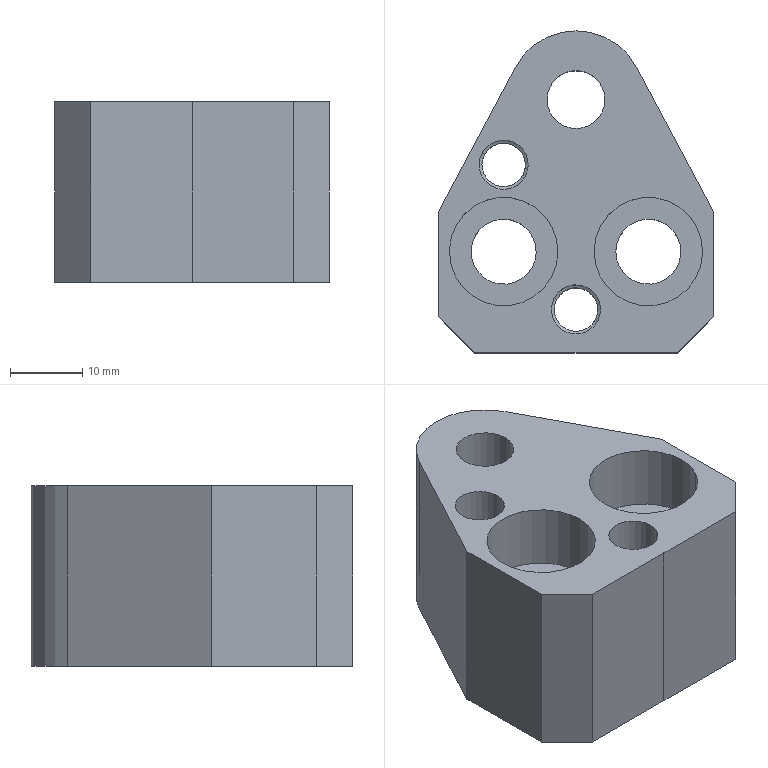Part | CATIA | 1 solid | 39 faces | box 38 x 44.5 x 25 mm | volume 24726 mm3 | cylinder 22 | plane 13 | cone 4 | commonest cylinder face diameters 6 x4 6.8 x4 9 x4 15 x4 8 x2 12 x2
STEP:
#1=CARTESIAN_POINT('',(2.984,-30.63,25.));
#2=VERTEX_POINT('',#1);
#3=CARTESIAN_POINT('',(-2.984,-27.37,25.));
#4=VERTEX_POINT('',#3);
#5=CARTESIAN_POINT('',(0.,-29.,25.));
#6=DIRECTION('',(0.,0.,-1.));
#7=AXIS2_PLACEMENT_3D('',#5,#6,$);
#8=CIRCLE('',#7,3.4);
#9=EDGE_CURVE('',#2,#4,#8,.F.);
#10=ORIENTED_EDGE('',*,*,#9,.T.);
#11=CARTESIAN_POINT('',(-2.984,-27.37,16.));
#12=VERTEX_POINT('',#11);
#13=CARTESIAN_POINT('',(-2.984,-27.37,20.655));
#14=DIRECTION('',(0.,0.,-1.));
#15=VECTOR('',#14,1.);
#16=LINE('',#13,#15);
#17=EDGE_CURVE('',#12,#4,#16,.F.);
#18=ORIENTED_EDGE('',*,*,#17,.F.);
#19=CARTESIAN_POINT('',(2.984,-30.63,16.));
#20=VERTEX_POINT('',#19);
#21=CARTESIAN_POINT('',(0.,-29.,16.));
#22=DIRECTION('',(0.,0.,-1.));
#23=AXIS2_PLACEMENT_3D('',#21,#22,$);
#24=CIRCLE('',#23,3.4);
#25=EDGE_CURVE('',#12,#20,#24,.T.);
#26=ORIENTED_EDGE('',*,*,#25,.T.);
#27=CARTESIAN_POINT('',(2.984,-30.63,20.655));
#28=DIRECTION('',(0.,0.,-1.));
#29=VECTOR('',#28,1.);
#30=LINE('',#27,#29);
#31=EDGE_CURVE('',#20,#2,#30,.F.);
#32=ORIENTED_EDGE('',*,*,#31,.T.);
#33=EDGE_LOOP('',(#10,#18,#26,#32));
#34=FACE_OUTER_BOUND('',#33,.T.);
#35=CARTESIAN_POINT('',(0.,-29.,24.9));
#36=DIRECTION('',(0.,0.,-1.));
#37=DIRECTION('',(0.8776,-0.4794,0.));
#38=AXIS2_PLACEMENT_3D('',#35,#36,#37);
#39=CYLINDRICAL_SURFACE('',#38,3.4);
#40=ADVANCED_FACE('',(#34),#39,.F.);
#41=CARTESIAN_POINT('',(0.,-29.,25.));
#42=DIRECTION('',(0.,0.,-1.));
#43=AXIS2_PLACEMENT_3D('',#41,#42,$);
#44=CIRCLE('',#43,3.4);
#45=EDGE_CURVE('',#4,#2,#44,.F.);
#46=ORIENTED_EDGE('',*,*,#45,.T.);
#47=ORIENTED_EDGE('',*,*,#31,.F.);
#48=CARTESIAN_POINT('',(0.,-29.,16.));
#49=DIRECTION('',(0.,0.,-1.));
#50=AXIS2_PLACEMENT_3D('',#48,#49,$);
#51=CIRCLE('',#50,3.4);
#52=EDGE_CURVE('',#20,#12,#51,.T.);
#53=ORIENTED_EDGE('',*,*,#52,.T.);
#54=ORIENTED_EDGE('',*,*,#17,.T.);
#55=EDGE_LOOP('',(#46,#47,#53,#54));
#56=FACE_OUTER_BOUND('',#55,.T.);
#57=ADVANCED_FACE('',(#56),#39,.F.);
#58=CARTESIAN_POINT('',(-2.633,-27.562,15.769));
#59=VERTEX_POINT('',#58);
#60=CARTESIAN_POINT('',(3.,-29.,15.769));
#61=VERTEX_POINT('',#60);
#62=CARTESIAN_POINT('',(0.,-29.,15.769));
#63=DIRECTION('',(0.,0.,1.));
#64=AXIS2_PLACEMENT_3D('',#62,#63,$);
#65=CIRCLE('',#64,3.);
#66=EDGE_CURVE('',#59,#61,#65,.F.);
#67=ORIENTED_EDGE('',*,*,#66,.T.);
#68=CARTESIAN_POINT('',(2.633,-30.438,15.769));
#69=VERTEX_POINT('',#68);
#70=CARTESIAN_POINT('',(0.,-29.,15.769));
#71=DIRECTION('',(0.,0.,1.));
#72=AXIS2_PLACEMENT_3D('',#70,#71,$);
#73=CIRCLE('',#72,3.);
#74=EDGE_CURVE('',#69,#61,#73,.T.);
#75=ORIENTED_EDGE('',*,*,#74,.F.);
#76=CARTESIAN_POINT('',(1.492,-29.815,15.019));
#77=DIRECTION('',(0.76,-0.4152,0.5));
#78=VECTOR('',#77,1.);
#79=LINE('',#76,#78);
#80=EDGE_CURVE('',#69,#20,#79,.T.);
#81=ORIENTED_EDGE('',*,*,#80,.T.);
#82=ORIENTED_EDGE('',*,*,#25,.F.);
#83=CARTESIAN_POINT('',(-1.492,-28.185,15.019));
#84=DIRECTION('',(-0.76,0.4152,0.5));
#85=VECTOR('',#84,1.);
#86=LINE('',#83,#85);
#87=EDGE_CURVE('',#59,#12,#86,.T.);
#88=ORIENTED_EDGE('',*,*,#87,.F.);
#89=EDGE_LOOP('',(#67,#75,#81,#82,#88));
#90=FACE_OUTER_BOUND('',#89,.T.);
#91=CARTESIAN_POINT('',(0.,-29.,14.037));
#92=DIRECTION('',(0.,0.,1.));
#93=DIRECTION('',(0.8776,-0.4794,0.));
#94=AXIS2_PLACEMENT_3D('',#91,#92,#93);
#95=CONICAL_SURFACE('',#94,0.,1.047);
#96=ADVANCED_FACE('',(#90),#95,.F.);
#97=CARTESIAN_POINT('',(-3.,-29.,15.769));
#98=VERTEX_POINT('',#97);
#99=CARTESIAN_POINT('',(0.,-29.,15.769));
#100=DIRECTION('',(0.,0.,1.));
#101=AXIS2_PLACEMENT_3D('',#99,#100,$);
#102=CIRCLE('',#101,3.);
#103=EDGE_CURVE('',#69,#98,#102,.F.);
#104=ORIENTED_EDGE('',*,*,#103,.T.);
#105=CARTESIAN_POINT('',(0.,-29.,15.769));
#106=DIRECTION('',(0.,0.,1.));
#107=AXIS2_PLACEMENT_3D('',#105,#106,$);
#108=CIRCLE('',#107,3.);
#109=EDGE_CURVE('',#59,#98,#108,.T.);
#110=ORIENTED_EDGE('',*,*,#109,.F.);
#111=ORIENTED_EDGE('',*,*,#87,.T.);
#112=ORIENTED_EDGE('',*,*,#52,.F.);
#113=ORIENTED_EDGE('',*,*,#80,.F.);
#114=EDGE_LOOP('',(#104,#110,#111,#112,#113));
#115=FACE_OUTER_BOUND('',#114,.T.);
#116=ADVANCED_FACE('',(#115),#95,.F.);
#117=ORIENTED_EDGE('',*,*,#66,.F.);
#118=ORIENTED_EDGE('',*,*,#109,.T.);
#119=CARTESIAN_POINT('',(-3.,-29.,0.));
#120=VERTEX_POINT('',#119);
#121=CARTESIAN_POINT('',(-3.,-29.,12.5));
#122=DIRECTION('',(0.,0.,1.));
#123=VECTOR('',#122,1.);
#124=LINE('',#121,#123);
#125=EDGE_CURVE('',#120,#98,#124,.T.);
#126=ORIENTED_EDGE('',*,*,#125,.F.);
#127=CARTESIAN_POINT('',(3.,-29.,0.));
#128=VERTEX_POINT('',#127);
#129=CARTESIAN_POINT('',(0.,-29.,0.));
#130=DIRECTION('',(0.,0.,1.));
#131=AXIS2_PLACEMENT_3D('',#129,#130,$);
#132=CIRCLE('',#131,3.);
#133=EDGE_CURVE('',#128,#120,#132,.T.);
#134=ORIENTED_EDGE('',*,*,#133,.F.);
#135=CARTESIAN_POINT('',(3.,-29.,12.5));
#136=DIRECTION('',(0.,0.,1.));
#137=VECTOR('',#136,1.);
#138=LINE('',#135,#137);
#139=EDGE_CURVE('',#128,#61,#138,.T.);
#140=ORIENTED_EDGE('',*,*,#139,.T.);
#141=EDGE_LOOP('',(#117,#118,#126,#134,#140));
#142=FACE_OUTER_BOUND('',#141,.T.);
#143=CARTESIAN_POINT('',(0.,-29.,12.5));
#144=DIRECTION('',(0.,0.,1.));
#145=DIRECTION('',(1.,0.,0.));
#146=AXIS2_PLACEMENT_3D('',#143,#144,#145);
#147=CYLINDRICAL_SURFACE('',#146,3.);
#148=ADVANCED_FACE('',(#142),#147,.F.);
#149=CARTESIAN_POINT('',(8.388,4.46,0.));
#150=VERTEX_POINT('',#149);
#151=CARTESIAN_POINT('',(8.388,4.46,25.));
#152=VERTEX_POINT('',#151);
#153=CARTESIAN_POINT('',(8.388,4.46,12.5));
#154=DIRECTION('',(0.,0.,1.));
#155=VECTOR('',#154,1.);
#156=LINE('',#153,#155);
#157=EDGE_CURVE('',#150,#152,#156,.T.);
#158=ORIENTED_EDGE('',*,*,#157,.F.);
#159=CARTESIAN_POINT('',(0.,9.5,0.));
#160=VERTEX_POINT('',#159);
#161=CARTESIAN_POINT('',(0.,0.,0.));
#162=DIRECTION('',(0.,0.,1.));
#163=AXIS2_PLACEMENT_3D('',#161,#162,$);
#164=CIRCLE('',#163,9.5);
#165=EDGE_CURVE('',#150,#160,#164,.T.);
#166=ORIENTED_EDGE('',*,*,#165,.T.);
#167=CARTESIAN_POINT('',(0.,9.5,25.));
#168=VERTEX_POINT('',#167);
#169=CARTESIAN_POINT('',(0.,9.5,12.5));
#170=DIRECTION('',(0.,0.,1.));
#171=VECTOR('',#170,1.);
#172=LINE('',#169,#171);
#173=EDGE_CURVE('',#160,#168,#172,.T.);
#174=ORIENTED_EDGE('',*,*,#173,.T.);
#175=CARTESIAN_POINT('',(0.,0.,25.));
#176=DIRECTION('',(0.,0.,1.));
#177=AXIS2_PLACEMENT_3D('',#175,#176,$);
#178=CIRCLE('',#177,9.5);
#179=EDGE_CURVE('',#152,#168,#178,.T.);
#180=ORIENTED_EDGE('',*,*,#179,.F.);
#181=EDGE_LOOP('',(#158,#166,#174,#180));
#182=FACE_OUTER_BOUND('',#181,.T.);
#183=CARTESIAN_POINT('',(0.,0.,12.5));
#184=DIRECTION('',(0.,0.,1.));
#185=DIRECTION('',(0.8829,0.4695,0.));
#186=AXIS2_PLACEMENT_3D('',#183,#184,#185);
#187=CYLINDRICAL_SURFACE('',#186,9.5);
#188=ADVANCED_FACE('',(#182),#187,.T.);
#189=ORIENTED_EDGE('',*,*,#173,.F.);
#190=CARTESIAN_POINT('',(-8.388,4.46,0.));
#191=VERTEX_POINT('',#190);
#192=CARTESIAN_POINT('',(0.,0.,0.));
#193=DIRECTION('',(0.,0.,1.));
#194=AXIS2_PLACEMENT_3D('',#192,#193,$);
#195=CIRCLE('',#194,9.5);
#196=EDGE_CURVE('',#160,#191,#195,.T.);
#197=ORIENTED_EDGE('',*,*,#196,.T.);
#198=CARTESIAN_POINT('',(-8.388,4.46,25.));
#199=VERTEX_POINT('',#198);
#200=CARTESIAN_POINT('',(-8.388,4.46,12.5));
#201=DIRECTION('',(0.,0.,1.));
#202=VECTOR('',#201,1.);
#203=LINE('',#200,#202);
#204=EDGE_CURVE('',#191,#199,#203,.T.);
#205=ORIENTED_EDGE('',*,*,#204,.T.);
#206=CARTESIAN_POINT('',(0.,0.,25.));
#207=DIRECTION('',(0.,0.,1.));
#208=AXIS2_PLACEMENT_3D('',#206,#207,$);
#209=CIRCLE('',#208,9.5);
#210=EDGE_CURVE('',#168,#199,#209,.T.);
#211=ORIENTED_EDGE('',*,*,#210,.F.);
#212=EDGE_LOOP('',(#189,#197,#205,#211));
#213=FACE_OUTER_BOUND('',#212,.T.);
#214=ADVANCED_FACE('',(#213),#187,.T.);
#215=ORIENTED_EDGE('',*,*,#204,.F.);
#216=CARTESIAN_POINT('',(-19.,-15.498,0.));
#217=VERTEX_POINT('',#216);
#218=CARTESIAN_POINT('',(-13.694,-5.519,0.));
#219=DIRECTION('',(-0.4695,-0.8829,0.));
#220=VECTOR('',#219,1.);
#221=LINE('',#218,#220);
#222=EDGE_CURVE('',#191,#217,#221,.T.);
#223=ORIENTED_EDGE('',*,*,#222,.T.);
#224=CARTESIAN_POINT('',(-19.,-15.498,25.));
#225=VERTEX_POINT('',#224);
#226=CARTESIAN_POINT('',(-19.,-15.498,12.5));
#227=DIRECTION('',(0.,0.,1.));
#228=VECTOR('',#227,1.);
#229=LINE('',#226,#228);
#230=EDGE_CURVE('',#217,#225,#229,.T.);
#231=ORIENTED_EDGE('',*,*,#230,.T.);
#232=CARTESIAN_POINT('',(-13.694,-5.519,25.));
#233=DIRECTION('',(-0.4695,-0.8829,0.));
#234=VECTOR('',#233,1.);
#235=LINE('',#232,#234);
#236=EDGE_CURVE('',#199,#225,#235,.T.);
#237=ORIENTED_EDGE('',*,*,#236,.F.);
#238=EDGE_LOOP('',(#215,#223,#231,#237));
#239=FACE_OUTER_BOUND('',#238,.T.);
#240=CARTESIAN_POINT('',(-8.388,4.46,0.));
#241=DIRECTION('',(-0.8829,0.4695,0.));
#242=DIRECTION('',(-0.4695,-0.8829,0.));
#243=AXIS2_PLACEMENT_3D('',#240,#241,#242);
#244=PLANE('',#243);
#245=ADVANCED_FACE('',(#239),#244,.T.);
#246=ORIENTED_EDGE('',*,*,#230,.F.);
#247=CARTESIAN_POINT('',(-19.,-30.,0.));
#248=VERTEX_POINT('',#247);
#249=CARTESIAN_POINT('',(-19.,-22.749,0.));
#250=DIRECTION('',(0.,-1.,0.));
#251=VECTOR('',#250,1.);
#252=LINE('',#249,#251);
#253=EDGE_CURVE('',#217,#248,#252,.T.);
#254=ORIENTED_EDGE('',*,*,#253,.T.);
#255=CARTESIAN_POINT('',(-19.,-30.,25.));
#256=VERTEX_POINT('',#255);
#257=CARTESIAN_POINT('',(-19.,-30.,12.5));
#258=DIRECTION('',(0.,0.,1.));
#259=VECTOR('',#258,1.);
#260=LINE('',#257,#259);
#261=EDGE_CURVE('',#248,#256,#260,.T.);
#262=ORIENTED_EDGE('',*,*,#261,.T.);
#263=CARTESIAN_POINT('',(-19.,-22.749,25.));
#264=DIRECTION('',(0.,-1.,0.));
#265=VECTOR('',#264,1.);
#266=LINE('',#263,#265);
#267=EDGE_CURVE('',#225,#256,#266,.T.);
#268=ORIENTED_EDGE('',*,*,#267,.F.);
#269=EDGE_LOOP('',(#246,#254,#262,#268));
#270=FACE_OUTER_BOUND('',#269,.T.);
#271=CARTESIAN_POINT('',(-19.,-15.498,0.));
#272=DIRECTION('',(-1.,0.,0.));
#273=DIRECTION('',(0.,-1.,0.));
#274=AXIS2_PLACEMENT_3D('',#271,#272,#273);
#275=PLANE('',#274);
#276=ADVANCED_FACE('',(#270),#275,.T.);
#277=ORIENTED_EDGE('',*,*,#261,.F.);
#278=CARTESIAN_POINT('',(-14.,-35.,0.));
#279=VERTEX_POINT('',#278);
#280=CARTESIAN_POINT('',(-16.5,-32.5,0.));
#281=DIRECTION('',(0.7071,-0.7071,0.));
#282=VECTOR('',#281,1.);
#283=LINE('',#280,#282);
#284=EDGE_CURVE('',#248,#279,#283,.T.);
#285=ORIENTED_EDGE('',*,*,#284,.T.);
#286=CARTESIAN_POINT('',(-14.,-35.,25.));
#287=VERTEX_POINT('',#286);
#288=CARTESIAN_POINT('',(-14.,-35.,12.5));
#289=DIRECTION('',(0.,0.,1.));
#290=VECTOR('',#289,1.);
#291=LINE('',#288,#290);
#292=EDGE_CURVE('',#279,#287,#291,.T.);
#293=ORIENTED_EDGE('',*,*,#292,.T.);
#294=CARTESIAN_POINT('',(-16.5,-32.5,25.));
#295=DIRECTION('',(0.7071,-0.7071,0.));
#296=VECTOR('',#295,1.);
#297=LINE('',#294,#296);
#298=EDGE_CURVE('',#256,#287,#297,.T.);
#299=ORIENTED_EDGE('',*,*,#298,.F.);
#300=EDGE_LOOP('',(#277,#285,#293,#299));
#301=FACE_OUTER_BOUND('',#300,.T.);
#302=CARTESIAN_POINT('',(-19.,-30.,0.));
#303=DIRECTION('',(-0.7071,-0.7071,0.));
#304=DIRECTION('',(0.7071,-0.7071,0.));
#305=AXIS2_PLACEMENT_3D('',#302,#303,#304);
#306=PLANE('',#305);
#307=ADVANCED_FACE('',(#301),#306,.T.);
#308=ORIENTED_EDGE('',*,*,#292,.F.);
#309=CARTESIAN_POINT('',(0.,-35.,0.));
#310=VERTEX_POINT('',#309);
#311=CARTESIAN_POINT('',(-7.,-35.,0.));
#312=DIRECTION('',(1.,0.,0.));
#313=VECTOR('',#312,1.);
#314=LINE('',#311,#313);
#315=EDGE_CURVE('',#279,#310,#314,.T.);
#316=ORIENTED_EDGE('',*,*,#315,.T.);
#317=CARTESIAN_POINT('',(0.,-35.,25.));
#318=VERTEX_POINT('',#317);
#319=CARTESIAN_POINT('',(0.,-35.,12.5));
#320=DIRECTION('',(0.,0.,1.));
#321=VECTOR('',#320,1.);
#322=LINE('',#319,#321);
#323=EDGE_CURVE('',#310,#318,#322,.T.);
#324=ORIENTED_EDGE('',*,*,#323,.T.);
#325=CARTESIAN_POINT('',(-7.,-35.,25.));
#326=DIRECTION('',(1.,0.,0.));
#327=VECTOR('',#326,1.);
#328=LINE('',#325,#327);
#329=EDGE_CURVE('',#287,#318,#328,.T.);
#330=ORIENTED_EDGE('',*,*,#329,.F.);
#331=EDGE_LOOP('',(#308,#316,#324,#330));
#332=FACE_OUTER_BOUND('',#331,.T.);
#333=CARTESIAN_POINT('',(-14.,-35.,0.));
#334=DIRECTION('',(0.,-1.,0.));
#335=DIRECTION('',(1.,0.,0.));
#336=AXIS2_PLACEMENT_3D('',#333,#334,#335);
#337=PLANE('',#336);
#338=ADVANCED_FACE('',(#332),#337,.T.);
#339=ORIENTED_EDGE('',*,*,#323,.F.);
#340=CARTESIAN_POINT('',(14.,-35.,0.));
#341=VERTEX_POINT('',#340);
#342=CARTESIAN_POINT('',(7.,-35.,0.));
#343=DIRECTION('',(-1.,0.,0.));
#344=VECTOR('',#343,1.);
#345=LINE('',#342,#344);
#346=EDGE_CURVE('',#310,#341,#345,.F.);
#347=ORIENTED_EDGE('',*,*,#346,.T.);
#348=CARTESIAN_POINT('',(14.,-35.,25.));
#349=VERTEX_POINT('',#348);
#350=CARTESIAN_POINT('',(14.,-35.,12.5));
#351=DIRECTION('',(0.,0.,1.));
#352=VECTOR('',#351,1.);
#353=LINE('',#350,#352);
#354=EDGE_CURVE('',#341,#349,#353,.T.);
#355=ORIENTED_EDGE('',*,*,#354,.T.);
#356=CARTESIAN_POINT('',(7.,-35.,25.));
#357=DIRECTION('',(-1.,0.,0.));
#358=VECTOR('',#357,1.);
#359=LINE('',#356,#358);
#360=EDGE_CURVE('',#318,#349,#359,.F.);
#361=ORIENTED_EDGE('',*,*,#360,.F.);
#362=EDGE_LOOP('',(#339,#347,#355,#361));
#363=FACE_OUTER_BOUND('',#362,.T.);
#364=ADVANCED_FACE('',(#363),#337,.T.);
#365=ORIENTED_EDGE('',*,*,#354,.F.);
#366=CARTESIAN_POINT('',(19.,-30.,0.));
#367=VERTEX_POINT('',#366);
#368=CARTESIAN_POINT('',(16.5,-32.5,0.));
#369=DIRECTION('',(-0.7071,-0.7071,0.));
#370=VECTOR('',#369,1.);
#371=LINE('',#368,#370);
#372=EDGE_CURVE('',#341,#367,#371,.F.);
#373=ORIENTED_EDGE('',*,*,#372,.T.);
#374=CARTESIAN_POINT('',(19.,-30.,25.));
#375=VERTEX_POINT('',#374);
#376=CARTESIAN_POINT('',(19.,-30.,12.5));
#377=DIRECTION('',(0.,0.,1.));
#378=VECTOR('',#377,1.);
#379=LINE('',#376,#378);
#380=EDGE_CURVE('',#367,#375,#379,.T.);
#381=ORIENTED_EDGE('',*,*,#380,.T.);
#382=CARTESIAN_POINT('',(16.5,-32.5,25.));
#383=DIRECTION('',(-0.7071,-0.7071,0.));
#384=VECTOR('',#383,1.);
#385=LINE('',#382,#384);
#386=EDGE_CURVE('',#349,#375,#385,.F.);
#387=ORIENTED_EDGE('',*,*,#386,.F.);
#388=EDGE_LOOP('',(#365,#373,#381,#387));
#389=FACE_OUTER_BOUND('',#388,.T.);
#390=CARTESIAN_POINT('',(19.,-30.,0.));
#391=DIRECTION('',(-0.7071,0.7071,0.));
#392=DIRECTION('',(-0.7071,-0.7071,0.));
#393=AXIS2_PLACEMENT_3D('',#390,#391,#392);
#394=PLANE('',#393);
#395=ADVANCED_FACE('',(#389),#394,.F.);
#396=ORIENTED_EDGE('',*,*,#380,.F.);
#397=CARTESIAN_POINT('',(19.,-15.498,0.));
#398=VERTEX_POINT('',#397);
#399=CARTESIAN_POINT('',(19.,-22.749,0.));
#400=DIRECTION('',(0.,-1.,0.));
#401=VECTOR('',#400,1.);
#402=LINE('',#399,#401);
#403=EDGE_CURVE('',#367,#398,#402,.F.);
#404=ORIENTED_EDGE('',*,*,#403,.T.);
#405=CARTESIAN_POINT('',(19.,-15.498,25.));
#406=VERTEX_POINT('',#405);
#407=CARTESIAN_POINT('',(19.,-15.498,12.5));
#408=DIRECTION('',(0.,0.,1.));
#409=VECTOR('',#408,1.);
#410=LINE('',#407,#409);
#411=EDGE_CURVE('',#398,#406,#410,.T.);
#412=ORIENTED_EDGE('',*,*,#411,.T.);
#413=CARTESIAN_POINT('',(19.,-22.749,25.));
#414=DIRECTION('',(0.,-1.,0.));
#415=VECTOR('',#414,1.);
#416=LINE('',#413,#415);
#417=EDGE_CURVE('',#375,#406,#416,.F.);
#418=ORIENTED_EDGE('',*,*,#417,.F.);
#419=EDGE_LOOP('',(#396,#404,#412,#418));
#420=FACE_OUTER_BOUND('',#419,.T.);
#421=CARTESIAN_POINT('',(19.,-15.498,0.));
#422=DIRECTION('',(-1.,0.,0.));
#423=DIRECTION('',(0.,-1.,0.));
#424=AXIS2_PLACEMENT_3D('',#421,#422,#423);
#425=PLANE('',#424);
#426=ADVANCED_FACE('',(#420),#425,.F.);
#427=ORIENTED_EDGE('',*,*,#411,.F.);
#428=CARTESIAN_POINT('',(13.694,-5.519,0.));
#429=DIRECTION('',(0.4695,-0.8829,0.));
#430=VECTOR('',#429,1.);
#431=LINE('',#428,#430);
#432=EDGE_CURVE('',#398,#150,#431,.F.);
#433=ORIENTED_EDGE('',*,*,#432,.T.);
#434=ORIENTED_EDGE('',*,*,#157,.T.);
#435=CARTESIAN_POINT('',(13.694,-5.519,25.));
#436=DIRECTION('',(0.4695,-0.8829,0.));
#437=VECTOR('',#436,1.);
#438=LINE('',#435,#437);
#439=EDGE_CURVE('',#406,#152,#438,.F.);
#440=ORIENTED_EDGE('',*,*,#439,.F.);
#441=EDGE_LOOP('',(#427,#433,#434,#440));
#442=FACE_OUTER_BOUND('',#441,.T.);
#443=CARTESIAN_POINT('',(8.388,4.46,0.));
#444=DIRECTION('',(-0.8829,-0.4695,0.));
#445=DIRECTION('',(0.4695,-0.8829,0.));
#446=AXIS2_PLACEMENT_3D('',#443,#444,#445);
#447=PLANE('',#446);
#448=ADVANCED_FACE('',(#442),#447,.F.);
#449=CARTESIAN_POINT('',(16.582,-24.596,16.));
#450=VERTEX_POINT('',#449);
#451=CARTESIAN_POINT('',(3.418,-17.404,16.));
#452=VERTEX_POINT('',#451);
#453=CARTESIAN_POINT('',(10.,-21.,16.));
#454=DIRECTION('',(0.,0.,-1.));
#455=AXIS2_PLACEMENT_3D('',#453,#454,$);
#456=CIRCLE('',#455,7.5);
#457=EDGE_CURVE('',#450,#452,#456,.T.);
#458=ORIENTED_EDGE('',*,*,#457,.F.);
#459=CARTESIAN_POINT('',(10.,-21.,16.));
#460=DIRECTION('',(0.,0.,-1.));
#461=AXIS2_PLACEMENT_3D('',#459,#460,$);
#462=CIRCLE('',#461,7.5);
#463=EDGE_CURVE('',#452,#450,#462,.T.);
#464=ORIENTED_EDGE('',*,*,#463,.F.);
#465=EDGE_LOOP('',(#458,#464));
#466=FACE_OUTER_BOUND('',#465,.T.);
#467=CARTESIAN_POINT('',(6.051,-18.843,16.));
#468=VERTEX_POINT('',#467);
#469=CARTESIAN_POINT('',(13.949,-23.157,16.));
#470=VERTEX_POINT('',#469);
#471=CARTESIAN_POINT('',(10.,-21.,16.));
#472=DIRECTION('',(0.,0.,-1.));
#473=AXIS2_PLACEMENT_3D('',#471,#472,$);
#474=CIRCLE('',#473,4.5);
#475=EDGE_CURVE('',#468,#470,#474,.T.);
#476=ORIENTED_EDGE('',*,*,#475,.T.);
#477=CARTESIAN_POINT('',(10.,-21.,16.));
#478=DIRECTION('',(0.,0.,-1.));
#479=AXIS2_PLACEMENT_3D('',#477,#478,$);
#480=CIRCLE('',#479,4.5);
#481=EDGE_CURVE('',#470,#468,#480,.T.);
#482=ORIENTED_EDGE('',*,*,#481,.T.);
#483=EDGE_LOOP('',(#476,#482));
#484=FACE_BOUND('',#483,.T.);
#485=CARTESIAN_POINT('',(-5.5,-21.,16.));
#486=DIRECTION('',(0.,0.,-1.));
#487=DIRECTION('',(1.,0.,0.));
#488=AXIS2_PLACEMENT_3D('',#485,#486,#487);
#489=PLANE('',#488);
#490=ADVANCED_FACE('',(#466,#484),#489,.F.);
#491=CARTESIAN_POINT('',(6.051,-18.843,0.));
#492=VERTEX_POINT('',#491);
#493=CARTESIAN_POINT('',(13.949,-23.157,0.));
#494=VERTEX_POINT('',#493);
#495=CARTESIAN_POINT('',(10.,-21.,0.));
#496=DIRECTION('',(0.,0.,-1.));
#497=AXIS2_PLACEMENT_3D('',#495,#496,$);
#498=CIRCLE('',#497,4.5);
#499=EDGE_CURVE('',#492,#494,#498,.F.);
#500=ORIENTED_EDGE('',*,*,#499,.F.);
#501=CARTESIAN_POINT('',(6.051,-18.843,7.8));
#502=DIRECTION('',(0.,0.,-1.));
#503=VECTOR('',#502,1.);
#504=LINE('',#501,#503);
#505=EDGE_CURVE('',#492,#468,#504,.F.);
#506=ORIENTED_EDGE('',*,*,#505,.T.);
#507=ORIENTED_EDGE('',*,*,#481,.F.);
#508=CARTESIAN_POINT('',(13.949,-23.157,7.8));
#509=DIRECTION('',(0.,0.,-1.));
#510=VECTOR('',#509,1.);
#511=LINE('',#508,#510);
#512=EDGE_CURVE('',#494,#470,#511,.F.);
#513=ORIENTED_EDGE('',*,*,#512,.F.);
#514=EDGE_LOOP('',(#500,#506,#507,#513));
#515=FACE_OUTER_BOUND('',#514,.T.);
#516=CARTESIAN_POINT('',(10.,-21.,24.9));
#517=DIRECTION('',(0.,0.,-1.));
#518=DIRECTION('',(0.8776,-0.4794,0.));
#519=AXIS2_PLACEMENT_3D('',#516,#517,#518);
#520=CYLINDRICAL_SURFACE('',#519,4.5);
#521=ADVANCED_FACE('',(#515),#520,.F.);
#522=CARTESIAN_POINT('',(10.,-21.,0.));
#523=DIRECTION('',(0.,0.,-1.));
#524=AXIS2_PLACEMENT_3D('',#522,#523,$);
#525=CIRCLE('',#524,4.5);
#526=EDGE_CURVE('',#494,#492,#525,.F.);
#527=ORIENTED_EDGE('',*,*,#526,.F.);
#528=ORIENTED_EDGE('',*,*,#512,.T.);
#529=ORIENTED_EDGE('',*,*,#475,.F.);
#530=ORIENTED_EDGE('',*,*,#505,.F.);
#531=EDGE_LOOP('',(#527,#528,#529,#530));
#532=FACE_OUTER_BOUND('',#531,.T.);
#533=ADVANCED_FACE('',(#532),#520,.F.);
#534=CARTESIAN_POINT('',(-3.418,-24.596,16.));
#535=VERTEX_POINT('',#534);
#536=CARTESIAN_POINT('',(-16.582,-17.404,16.));
#537=VERTEX_POINT('',#536);
#538=CARTESIAN_POINT('',(-10.,-21.,16.));
#539=DIRECTION('',(0.,0.,-1.));
#540=AXIS2_PLACEMENT_3D('',#538,#539,$);
#541=CIRCLE('',#540,7.5);
#542=EDGE_CURVE('',#535,#537,#541,.T.);
#543=ORIENTED_EDGE('',*,*,#542,.F.);
#544=CARTESIAN_POINT('',(-10.,-21.,16.));
#545=DIRECTION('',(0.,0.,-1.));
#546=AXIS2_PLACEMENT_3D('',#544,#545,$);
#547=CIRCLE('',#546,7.5);
#548=EDGE_CURVE('',#537,#535,#547,.T.);
#549=ORIENTED_EDGE('',*,*,#548,.F.);
#550=EDGE_LOOP('',(#543,#549));
#551=FACE_OUTER_BOUND('',#550,.T.);
#552=CARTESIAN_POINT('',(-13.949,-18.843,16.));
#553=VERTEX_POINT('',#552);
#554=CARTESIAN_POINT('',(-6.051,-23.157,16.));
#555=VERTEX_POINT('',#554);
#556=CARTESIAN_POINT('',(-10.,-21.,16.));
#557=DIRECTION('',(0.,0.,-1.));
#558=AXIS2_PLACEMENT_3D('',#556,#557,$);
#559=CIRCLE('',#558,4.5);
#560=EDGE_CURVE('',#553,#555,#559,.T.);
#561=ORIENTED_EDGE('',*,*,#560,.T.);
#562=CARTESIAN_POINT('',(-10.,-21.,16.));
#563=DIRECTION('',(0.,0.,-1.));
#564=AXIS2_PLACEMENT_3D('',#562,#563,$);
#565=CIRCLE('',#564,4.5);
#566=EDGE_CURVE('',#555,#553,#565,.T.);
#567=ORIENTED_EDGE('',*,*,#566,.T.);
#568=EDGE_LOOP('',(#561,#567));
#569=FACE_BOUND('',#568,.T.);
#570=ADVANCED_FACE('',(#551,#569),#489,.F.);
#571=CARTESIAN_POINT('',(-13.949,-18.843,0.));
#572=VERTEX_POINT('',#571);
#573=CARTESIAN_POINT('',(-6.051,-23.157,0.));
#574=VERTEX_POINT('',#573);
#575=CARTESIAN_POINT('',(-10.,-21.,0.));
#576=DIRECTION('',(0.,0.,-1.));
#577=AXIS2_PLACEMENT_3D('',#575,#576,$);
#578=CIRCLE('',#577,4.5);
#579=EDGE_CURVE('',#572,#574,#578,.F.);
#580=ORIENTED_EDGE('',*,*,#579,.F.);
#581=CARTESIAN_POINT('',(-13.949,-18.843,7.8));
#582=DIRECTION('',(0.,0.,-1.));
#583=VECTOR('',#582,1.);
#584=LINE('',#581,#583);
#585=EDGE_CURVE('',#572,#553,#584,.F.);
#586=ORIENTED_EDGE('',*,*,#585,.T.);
#587=ORIENTED_EDGE('',*,*,#566,.F.);
#588=CARTESIAN_POINT('',(-6.051,-23.157,7.8));
#589=DIRECTION('',(0.,0.,-1.));
#590=VECTOR('',#589,1.);
#591=LINE('',#588,#590);
#592=EDGE_CURVE('',#574,#555,#591,.F.);
#593=ORIENTED_EDGE('',*,*,#592,.F.);
#594=EDGE_LOOP('',(#580,#586,#587,#593));
#595=FACE_OUTER_BOUND('',#594,.T.);
#596=CARTESIAN_POINT('',(-10.,-21.,24.9));
#597=DIRECTION('',(0.,0.,-1.));
#598=DIRECTION('',(0.8776,-0.4794,0.));
#599=AXIS2_PLACEMENT_3D('',#596,#597,#598);
#600=CYLINDRICAL_SURFACE('',#599,4.5);
#601=ADVANCED_FACE('',(#595),#600,.F.);
#602=CARTESIAN_POINT('',(-10.,-21.,0.));
#603=DIRECTION('',(0.,0.,-1.));
#604=AXIS2_PLACEMENT_3D('',#602,#603,$);
#605=CIRCLE('',#604,4.5);
#606=EDGE_CURVE('',#574,#572,#605,.F.);
#607=ORIENTED_EDGE('',*,*,#606,.F.);
#608=ORIENTED_EDGE('',*,*,#592,.T.);
#609=ORIENTED_EDGE('',*,*,#560,.F.);
#610=ORIENTED_EDGE('',*,*,#585,.F.);
#611=EDGE_LOOP('',(#607,#608,#609,#610));
#612=FACE_OUTER_BOUND('',#611,.T.);
#613=ADVANCED_FACE('',(#612),#600,.F.);
#614=CARTESIAN_POINT('',(6.,0.,5.));
#615=VERTEX_POINT('',#614);
#616=CARTESIAN_POINT('',(-6.,0.,5.));
#617=VERTEX_POINT('',#616);
#618=CARTESIAN_POINT('',(0.,0.,5.));
#619=DIRECTION('',(0.,0.,1.));
#620=AXIS2_PLACEMENT_3D('',#618,#619,$);
#621=CIRCLE('',#620,6.);
#622=EDGE_CURVE('',#615,#617,#621,.T.);
#623=ORIENTED_EDGE('',*,*,#622,.T.);
#624=CARTESIAN_POINT('',(-6.,0.,0.));
#625=VERTEX_POINT('',#624);
#626=CARTESIAN_POINT('',(-6.,0.,2.5));
#627=DIRECTION('',(0.,0.,1.));
#628=VECTOR('',#627,1.);
#629=LINE('',#626,#628);
#630=EDGE_CURVE('',#625,#617,#629,.T.);
#631=ORIENTED_EDGE('',*,*,#630,.F.);
#632=CARTESIAN_POINT('',(6.,0.,0.));
#633=VERTEX_POINT('',#632);
#634=CARTESIAN_POINT('',(0.,0.,0.));
#635=DIRECTION('',(0.,0.,1.));
#636=AXIS2_PLACEMENT_3D('',#634,#635,$);
#637=CIRCLE('',#636,6.);
#638=EDGE_CURVE('',#633,#625,#637,.T.);
#639=ORIENTED_EDGE('',*,*,#638,.F.);
#640=CARTESIAN_POINT('',(6.,0.,2.5));
#641=DIRECTION('',(0.,0.,1.));
#642=VECTOR('',#641,1.);
#643=LINE('',#640,#642);
#644=EDGE_CURVE('',#633,#615,#643,.T.);
#645=ORIENTED_EDGE('',*,*,#644,.T.);
#646=EDGE_LOOP('',(#623,#631,#639,#645));
#647=FACE_OUTER_BOUND('',#646,.T.);
#648=CARTESIAN_POINT('',(0.,0.,2.5));
#649=DIRECTION('',(0.,0.,1.));
#650=DIRECTION('',(1.,0.,0.));
#651=AXIS2_PLACEMENT_3D('',#648,#649,#650);
#652=CYLINDRICAL_SURFACE('',#651,6.);
#653=ADVANCED_FACE('',(#647),#652,.F.);
#654=CARTESIAN_POINT('',(0.,0.,5.));
#655=DIRECTION('',(0.,0.,1.));
#656=AXIS2_PLACEMENT_3D('',#654,#655,$);
#657=CIRCLE('',#656,6.);
#658=EDGE_CURVE('',#617,#615,#657,.T.);
#659=ORIENTED_EDGE('',*,*,#658,.T.);
#660=ORIENTED_EDGE('',*,*,#644,.F.);
#661=CARTESIAN_POINT('',(0.,0.,0.));
#662=DIRECTION('',(0.,0.,1.));
#663=AXIS2_PLACEMENT_3D('',#661,#662,$);
#664=CIRCLE('',#663,6.);
#665=EDGE_CURVE('',#625,#633,#664,.T.);
#666=ORIENTED_EDGE('',*,*,#665,.F.);
#667=ORIENTED_EDGE('',*,*,#630,.T.);
#668=EDGE_LOOP('',(#659,#660,#666,#667));
#669=FACE_OUTER_BOUND('',#668,.T.);
#670=ADVANCED_FACE('',(#669),#652,.F.);
#671=ORIENTED_EDGE('',*,*,#658,.F.);
#672=ORIENTED_EDGE('',*,*,#622,.F.);
#673=EDGE_LOOP('',(#671,#672));
#674=FACE_OUTER_BOUND('',#673,.T.);
#675=CARTESIAN_POINT('',(4.,0.,5.));
#676=VERTEX_POINT('',#675);
#677=CARTESIAN_POINT('',(-4.,0.,5.));
#678=VERTEX_POINT('',#677);
#679=CARTESIAN_POINT('',(0.,0.,5.));
#680=DIRECTION('',(0.,0.,1.));
#681=AXIS2_PLACEMENT_3D('',#679,#680,$);
#682=CIRCLE('',#681,4.);
#683=EDGE_CURVE('',#676,#678,#682,.T.);
#684=ORIENTED_EDGE('',*,*,#683,.T.);
#685=CARTESIAN_POINT('',(0.,0.,5.));
#686=DIRECTION('',(0.,0.,1.));
#687=AXIS2_PLACEMENT_3D('',#685,#686,$);
#688=CIRCLE('',#687,4.);
#689=EDGE_CURVE('',#678,#676,#688,.T.);
#690=ORIENTED_EDGE('',*,*,#689,.T.);
#691=EDGE_LOOP('',(#684,#690));
#692=FACE_BOUND('',#691,.T.);
#693=CARTESIAN_POINT('',(0.,0.,5.));
#694=DIRECTION('',(0.,0.,1.));
#695=DIRECTION('',(1.,0.,0.));
#696=AXIS2_PLACEMENT_3D('',#693,#694,#695);
#697=PLANE('',#696);
#698=ADVANCED_FACE('',(#674,#692),#697,.F.);
#699=ORIENTED_EDGE('',*,*,#432,.F.);
#700=ORIENTED_EDGE('',*,*,#403,.F.);
#701=ORIENTED_EDGE('',*,*,#372,.F.);
#702=ORIENTED_EDGE('',*,*,#346,.F.);
#703=ORIENTED_EDGE('',*,*,#315,.F.);
#704=ORIENTED_EDGE('',*,*,#284,.F.);
#705=ORIENTED_EDGE('',*,*,#253,.F.);
#706=ORIENTED_EDGE('',*,*,#222,.F.);
#707=ORIENTED_EDGE('',*,*,#196,.F.);
#708=ORIENTED_EDGE('',*,*,#165,.F.);
#709=EDGE_LOOP('',(#699,#700,#701,#702,#703,#704,#705,#706,#707,#708));
#710=FACE_OUTER_BOUND('',#709,.T.);
#711=ORIENTED_EDGE('',*,*,#499,.T.);
#712=ORIENTED_EDGE('',*,*,#526,.T.);
#713=EDGE_LOOP('',(#711,#712));
#714=FACE_BOUND('',#713,.T.);
#715=ORIENTED_EDGE('',*,*,#579,.T.);
#716=ORIENTED_EDGE('',*,*,#606,.T.);
#717=EDGE_LOOP('',(#715,#716));
#718=FACE_BOUND('',#717,.T.);
#719=ORIENTED_EDGE('',*,*,#665,.T.);
#720=ORIENTED_EDGE('',*,*,#638,.T.);
#721=EDGE_LOOP('',(#719,#720));
#722=FACE_BOUND('',#721,.T.);
#723=ORIENTED_EDGE('',*,*,#133,.T.);
#724=CARTESIAN_POINT('',(0.,-29.,0.));
#725=DIRECTION('',(0.,0.,1.));
#726=AXIS2_PLACEMENT_3D('',#724,#725,$);
#727=CIRCLE('',#726,3.);
#728=EDGE_CURVE('',#120,#128,#727,.T.);
#729=ORIENTED_EDGE('',*,*,#728,.T.);
#730=EDGE_LOOP('',(#723,#729));
#731=FACE_BOUND('',#730,.T.);
#732=CARTESIAN_POINT('',(-7.,-9.,0.));
#733=VERTEX_POINT('',#732);
#734=CARTESIAN_POINT('',(-13.,-9.,0.));
#735=VERTEX_POINT('',#734);
#736=CARTESIAN_POINT('',(-10.,-9.,0.));
#737=DIRECTION('',(0.,0.,1.));
#738=AXIS2_PLACEMENT_3D('',#736,#737,$);
#739=CIRCLE('',#738,3.);
#740=EDGE_CURVE('',#733,#735,#739,.T.);
#741=ORIENTED_EDGE('',*,*,#740,.T.);
#742=CARTESIAN_POINT('',(-10.,-9.,0.));
#743=DIRECTION('',(0.,0.,1.));
#744=AXIS2_PLACEMENT_3D('',#742,#743,$);
#745=CIRCLE('',#744,3.);
#746=EDGE_CURVE('',#735,#733,#745,.T.);
#747=ORIENTED_EDGE('',*,*,#746,.T.);
#748=EDGE_LOOP('',(#741,#747));
#749=FACE_BOUND('',#748,.T.);
#750=CARTESIAN_POINT('',(0.,0.,0.));
#751=DIRECTION('',(0.,0.,1.));
#752=DIRECTION('',(1.,0.,0.));
#753=AXIS2_PLACEMENT_3D('',#750,#751,#752);
#754=PLANE('',#753);
#755=ADVANCED_FACE('',(#710,#714,#718,#722,#731,#749),#754,.F.);
#756=ORIENTED_EDGE('',*,*,#683,.F.);
#757=CARTESIAN_POINT('',(4.,0.,25.));
#758=VERTEX_POINT('',#757);
#759=CARTESIAN_POINT('',(4.,0.,12.5));
#760=DIRECTION('',(0.,0.,1.));
#761=VECTOR('',#760,1.);
#762=LINE('',#759,#761);
#763=EDGE_CURVE('',#676,#758,#762,.T.);
#764=ORIENTED_EDGE('',*,*,#763,.T.);
#765=CARTESIAN_POINT('',(-4.,0.,25.));
#766=VERTEX_POINT('',#765);
#767=CARTESIAN_POINT('',(0.,0.,25.));
#768=DIRECTION('',(0.,0.,1.));
#769=AXIS2_PLACEMENT_3D('',#767,#768,$);
#770=CIRCLE('',#769,4.);
#771=EDGE_CURVE('',#758,#766,#770,.T.);
#772=ORIENTED_EDGE('',*,*,#771,.T.);
#773=CARTESIAN_POINT('',(-4.,0.,12.5));
#774=DIRECTION('',(0.,0.,1.));
#775=VECTOR('',#774,1.);
#776=LINE('',#773,#775);
#777=EDGE_CURVE('',#678,#766,#776,.T.);
#778=ORIENTED_EDGE('',*,*,#777,.F.);
#779=EDGE_LOOP('',(#756,#764,#772,#778));
#780=FACE_OUTER_BOUND('',#779,.T.);
#781=CARTESIAN_POINT('',(0.,0.,12.5));
#782=DIRECTION('',(0.,0.,1.));
#783=DIRECTION('',(1.,0.,0.));
#784=AXIS2_PLACEMENT_3D('',#781,#782,#783);
#785=CYLINDRICAL_SURFACE('',#784,4.);
#786=ADVANCED_FACE('',(#780),#785,.F.);
#787=ORIENTED_EDGE('',*,*,#689,.F.);
#788=ORIENTED_EDGE('',*,*,#777,.T.);
#789=CARTESIAN_POINT('',(0.,0.,25.));
#790=DIRECTION('',(0.,0.,1.));
#791=AXIS2_PLACEMENT_3D('',#789,#790,$);
#792=CIRCLE('',#791,4.);
#793=EDGE_CURVE('',#766,#758,#792,.T.);
#794=ORIENTED_EDGE('',*,*,#793,.T.);
#795=ORIENTED_EDGE('',*,*,#763,.F.);
#796=EDGE_LOOP('',(#787,#788,#794,#795));
#797=FACE_OUTER_BOUND('',#796,.T.);
#798=ADVANCED_FACE('',(#797),#785,.F.);
#799=CARTESIAN_POINT('',(-3.418,-24.596,25.));
#800=VERTEX_POINT('',#799);
#801=CARTESIAN_POINT('',(-16.582,-17.404,25.));
#802=VERTEX_POINT('',#801);
#803=CARTESIAN_POINT('',(-10.,-21.,25.));
#804=DIRECTION('',(0.,0.,-1.));
#805=AXIS2_PLACEMENT_3D('',#803,#804,$);
#806=CIRCLE('',#805,7.5);
#807=EDGE_CURVE('',#800,#802,#806,.F.);
#808=ORIENTED_EDGE('',*,*,#807,.T.);
#809=CARTESIAN_POINT('',(-16.582,-17.404,20.655));
#810=DIRECTION('',(0.,0.,-1.));
#811=VECTOR('',#810,1.);
#812=LINE('',#809,#811);
#813=EDGE_CURVE('',#537,#802,#812,.F.);
#814=ORIENTED_EDGE('',*,*,#813,.F.);
#815=ORIENTED_EDGE('',*,*,#548,.T.);
#816=CARTESIAN_POINT('',(-3.418,-24.596,20.655));
#817=DIRECTION('',(0.,0.,-1.));
#818=VECTOR('',#817,1.);
#819=LINE('',#816,#818);
#820=EDGE_CURVE('',#535,#800,#819,.F.);
#821=ORIENTED_EDGE('',*,*,#820,.T.);
#822=EDGE_LOOP('',(#808,#814,#815,#821));
#823=FACE_OUTER_BOUND('',#822,.T.);
#824=CARTESIAN_POINT('',(-10.,-21.,24.9));
#825=DIRECTION('',(0.,0.,-1.));
#826=DIRECTION('',(0.8776,-0.4794,0.));
#827=AXIS2_PLACEMENT_3D('',#824,#825,#826);
#828=CYLINDRICAL_SURFACE('',#827,7.5);
#829=ADVANCED_FACE('',(#823),#828,.F.);
#830=CARTESIAN_POINT('',(-10.,-21.,25.));
#831=DIRECTION('',(0.,0.,-1.));
#832=AXIS2_PLACEMENT_3D('',#830,#831,$);
#833=CIRCLE('',#832,7.5);
#834=EDGE_CURVE('',#802,#800,#833,.F.);
#835=ORIENTED_EDGE('',*,*,#834,.T.);
#836=ORIENTED_EDGE('',*,*,#820,.F.);
#837=ORIENTED_EDGE('',*,*,#542,.T.);
#838=ORIENTED_EDGE('',*,*,#813,.T.);
#839=EDGE_LOOP('',(#835,#836,#837,#838));
#840=FACE_OUTER_BOUND('',#839,.T.);
#841=ADVANCED_FACE('',(#840),#828,.F.);
#842=CARTESIAN_POINT('',(3.418,-17.404,25.));
#843=VERTEX_POINT('',#842);
#844=CARTESIAN_POINT('',(16.582,-24.596,25.));
#845=VERTEX_POINT('',#844);
#846=CARTESIAN_POINT('',(10.,-21.,25.));
#847=DIRECTION('',(0.,0.,-1.));
#848=AXIS2_PLACEMENT_3D('',#846,#847,$);
#849=CIRCLE('',#848,7.5);
#850=EDGE_CURVE('',#843,#845,#849,.F.);
#851=ORIENTED_EDGE('',*,*,#850,.T.);
#852=CARTESIAN_POINT('',(16.582,-24.596,20.655));
#853=DIRECTION('',(0.,0.,-1.));
#854=VECTOR('',#853,1.);
#855=LINE('',#852,#854);
#856=EDGE_CURVE('',#450,#845,#855,.F.);
#857=ORIENTED_EDGE('',*,*,#856,.F.);
#858=ORIENTED_EDGE('',*,*,#457,.T.);
#859=CARTESIAN_POINT('',(3.418,-17.404,20.655));
#860=DIRECTION('',(0.,0.,-1.));
#861=VECTOR('',#860,1.);
#862=LINE('',#859,#861);
#863=EDGE_CURVE('',#452,#843,#862,.F.);
#864=ORIENTED_EDGE('',*,*,#863,.T.);
#865=EDGE_LOOP('',(#851,#857,#858,#864));
#866=FACE_OUTER_BOUND('',#865,.T.);
#867=CARTESIAN_POINT('',(10.,-21.,24.9));
#868=DIRECTION('',(0.,0.,-1.));
#869=DIRECTION('',(0.8776,-0.4794,0.));
#870=AXIS2_PLACEMENT_3D('',#867,#868,#869);
#871=CYLINDRICAL_SURFACE('',#870,7.5);
#872=ADVANCED_FACE('',(#866),#871,.F.);
#873=CARTESIAN_POINT('',(10.,-21.,25.));
#874=DIRECTION('',(0.,0.,-1.));
#875=AXIS2_PLACEMENT_3D('',#873,#874,$);
#876=CIRCLE('',#875,7.5);
#877=EDGE_CURVE('',#845,#843,#876,.F.);
#878=ORIENTED_EDGE('',*,*,#877,.T.);
#879=ORIENTED_EDGE('',*,*,#863,.F.);
#880=ORIENTED_EDGE('',*,*,#463,.T.);
#881=ORIENTED_EDGE('',*,*,#856,.T.);
#882=EDGE_LOOP('',(#878,#879,#880,#881));
#883=FACE_OUTER_BOUND('',#882,.T.);
#884=ADVANCED_FACE('',(#883),#871,.F.);
#885=ORIENTED_EDGE('',*,*,#103,.F.);
#886=ORIENTED_EDGE('',*,*,#74,.T.);
#887=ORIENTED_EDGE('',*,*,#139,.F.);
#888=ORIENTED_EDGE('',*,*,#728,.F.);
#889=ORIENTED_EDGE('',*,*,#125,.T.);
#890=EDGE_LOOP('',(#885,#886,#887,#888,#889));
#891=FACE_OUTER_BOUND('',#890,.T.);
#892=ADVANCED_FACE('',(#891),#147,.F.);
#893=CARTESIAN_POINT('',(-7.367,-10.438,15.769));
#894=VERTEX_POINT('',#893);
#895=CARTESIAN_POINT('',(-13.,-9.,15.769));
#896=VERTEX_POINT('',#895);
#897=CARTESIAN_POINT('',(-10.,-9.,15.769));
#898=DIRECTION('',(0.,0.,1.));
#899=AXIS2_PLACEMENT_3D('',#897,#898,$);
#900=CIRCLE('',#899,3.);
#901=EDGE_CURVE('',#894,#896,#900,.F.);
#902=ORIENTED_EDGE('',*,*,#901,.F.);
#903=CARTESIAN_POINT('',(-7.,-9.,15.769));
#904=VERTEX_POINT('',#903);
#905=CARTESIAN_POINT('',(-10.,-9.,15.769));
#906=DIRECTION('',(0.,0.,1.));
#907=AXIS2_PLACEMENT_3D('',#905,#906,$);
#908=CIRCLE('',#907,3.);
#909=EDGE_CURVE('',#894,#904,#908,.T.);
#910=ORIENTED_EDGE('',*,*,#909,.T.);
#911=CARTESIAN_POINT('',(-7.,-9.,12.5));
#912=DIRECTION('',(0.,0.,1.));
#913=VECTOR('',#912,1.);
#914=LINE('',#911,#913);
#915=EDGE_CURVE('',#733,#904,#914,.T.);
#916=ORIENTED_EDGE('',*,*,#915,.F.);
#917=ORIENTED_EDGE('',*,*,#746,.F.);
#918=CARTESIAN_POINT('',(-13.,-9.,12.5));
#919=DIRECTION('',(0.,0.,1.));
#920=VECTOR('',#919,1.);
#921=LINE('',#918,#920);
#922=EDGE_CURVE('',#735,#896,#921,.T.);
#923=ORIENTED_EDGE('',*,*,#922,.T.);
#924=EDGE_LOOP('',(#902,#910,#916,#917,#923));
#925=FACE_OUTER_BOUND('',#924,.T.);
#926=CARTESIAN_POINT('',(-10.,-9.,12.5));
#927=DIRECTION('',(0.,0.,1.));
#928=DIRECTION('',(1.,0.,0.));
#929=AXIS2_PLACEMENT_3D('',#926,#927,#928);
#930=CYLINDRICAL_SURFACE('',#929,3.);
#931=ADVANCED_FACE('',(#925),#930,.F.);
#932=CARTESIAN_POINT('',(-12.633,-7.562,15.769));
#933=VERTEX_POINT('',#932);
#934=CARTESIAN_POINT('',(-10.,-9.,15.769));
#935=DIRECTION('',(0.,0.,1.));
#936=AXIS2_PLACEMENT_3D('',#934,#935,$);
#937=CIRCLE('',#936,3.);
#938=EDGE_CURVE('',#933,#904,#937,.F.);
#939=ORIENTED_EDGE('',*,*,#938,.F.);
#940=CARTESIAN_POINT('',(-10.,-9.,15.769));
#941=DIRECTION('',(0.,0.,1.));
#942=AXIS2_PLACEMENT_3D('',#940,#941,$);
#943=CIRCLE('',#942,3.);
#944=EDGE_CURVE('',#933,#896,#943,.T.);
#945=ORIENTED_EDGE('',*,*,#944,.T.);
#946=ORIENTED_EDGE('',*,*,#922,.F.);
#947=ORIENTED_EDGE('',*,*,#740,.F.);
#948=ORIENTED_EDGE('',*,*,#915,.T.);
#949=EDGE_LOOP('',(#939,#945,#946,#947,#948));
#950=FACE_OUTER_BOUND('',#949,.T.);
#951=ADVANCED_FACE('',(#950),#930,.F.);
#952=ORIENTED_EDGE('',*,*,#179,.T.);
#953=ORIENTED_EDGE('',*,*,#210,.T.);
#954=ORIENTED_EDGE('',*,*,#236,.T.);
#955=ORIENTED_EDGE('',*,*,#267,.T.);
#956=ORIENTED_EDGE('',*,*,#298,.T.);
#957=ORIENTED_EDGE('',*,*,#329,.T.);
#958=ORIENTED_EDGE('',*,*,#360,.T.);
#959=ORIENTED_EDGE('',*,*,#386,.T.);
#960=ORIENTED_EDGE('',*,*,#417,.T.);
#961=ORIENTED_EDGE('',*,*,#439,.T.);
#962=EDGE_LOOP('',(#952,#953,#954,#955,#956,#957,#958,#959,#960,#961));
#963=FACE_OUTER_BOUND('',#962,.T.);
#964=CARTESIAN_POINT('',(-7.016,-10.63,25.));
#965=VERTEX_POINT('',#964);
#966=CARTESIAN_POINT('',(-12.984,-7.37,25.));
#967=VERTEX_POINT('',#966);
#968=CARTESIAN_POINT('',(-10.,-9.,25.));
#969=DIRECTION('',(0.,0.,1.));
#970=AXIS2_PLACEMENT_3D('',#968,#969,$);
#971=CIRCLE('',#970,3.4);
#972=EDGE_CURVE('',#965,#967,#971,.T.);
#973=ORIENTED_EDGE('',*,*,#972,.F.);
#974=CARTESIAN_POINT('',(-10.,-9.,25.));
#975=DIRECTION('',(0.,0.,1.));
#976=AXIS2_PLACEMENT_3D('',#974,#975,$);
#977=CIRCLE('',#976,3.4);
#978=EDGE_CURVE('',#967,#965,#977,.T.);
#979=ORIENTED_EDGE('',*,*,#978,.F.);
#980=EDGE_LOOP('',(#973,#979));
#981=FACE_BOUND('',#980,.T.);
#982=ORIENTED_EDGE('',*,*,#45,.F.);
#983=ORIENTED_EDGE('',*,*,#9,.F.);
#984=EDGE_LOOP('',(#982,#983));
#985=FACE_BOUND('',#984,.T.);
#986=ORIENTED_EDGE('',*,*,#877,.F.);
#987=ORIENTED_EDGE('',*,*,#850,.F.);
#988=EDGE_LOOP('',(#986,#987));
#989=FACE_BOUND('',#988,.T.);
#990=ORIENTED_EDGE('',*,*,#834,.F.);
#991=ORIENTED_EDGE('',*,*,#807,.F.);
#992=EDGE_LOOP('',(#990,#991));
#993=FACE_BOUND('',#992,.T.);
#994=ORIENTED_EDGE('',*,*,#793,.F.);
#995=ORIENTED_EDGE('',*,*,#771,.F.);
#996=EDGE_LOOP('',(#994,#995));
#997=FACE_BOUND('',#996,.T.);
#998=CARTESIAN_POINT('',(0.,0.,25.));
#999=DIRECTION('',(0.,0.,1.));
#1000=DIRECTION('',(1.,0.,0.));
#1001=AXIS2_PLACEMENT_3D('',#998,#999,#1000);
#1002=PLANE('',#1001);
#1003=ADVANCED_FACE('',(#963,#981,#985,#989,#993,#997),#1002,.T.);
#1004=ORIENTED_EDGE('',*,*,#972,.T.);
#1005=CARTESIAN_POINT('',(-12.984,-7.37,16.));
#1006=VERTEX_POINT('',#1005);
#1007=CARTESIAN_POINT('',(-12.984,-7.37,20.655));
#1008=DIRECTION('',(0.,0.,-1.));
#1009=VECTOR('',#1008,1.);
#1010=LINE('',#1007,#1009);
#1011=EDGE_CURVE('',#1006,#967,#1010,.F.);
#1012=ORIENTED_EDGE('',*,*,#1011,.F.);
#1013=CARTESIAN_POINT('',(-7.016,-10.63,16.));
#1014=VERTEX_POINT('',#1013);
#1015=CARTESIAN_POINT('',(-10.,-9.,16.));
#1016=DIRECTION('',(0.,0.,-1.));
#1017=AXIS2_PLACEMENT_3D('',#1015,#1016,$);
#1018=CIRCLE('',#1017,3.4);
#1019=EDGE_CURVE('',#1006,#1014,#1018,.T.);
#1020=ORIENTED_EDGE('',*,*,#1019,.T.);
#1021=CARTESIAN_POINT('',(-7.016,-10.63,20.655));
#1022=DIRECTION('',(0.,0.,-1.));
#1023=VECTOR('',#1022,1.);
#1024=LINE('',#1021,#1023);
#1025=EDGE_CURVE('',#1014,#965,#1024,.F.);
#1026=ORIENTED_EDGE('',*,*,#1025,.T.);
#1027=EDGE_LOOP('',(#1004,#1012,#1020,#1026));
#1028=FACE_OUTER_BOUND('',#1027,.T.);
#1029=CARTESIAN_POINT('',(-10.,-9.,24.9));
#1030=DIRECTION('',(0.,0.,-1.));
#1031=DIRECTION('',(0.8776,-0.4794,0.));
#1032=AXIS2_PLACEMENT_3D('',#1029,#1030,#1031);
#1033=CYLINDRICAL_SURFACE('',#1032,3.4);
#1034=ADVANCED_FACE('',(#1028),#1033,.F.);
#1035=ORIENTED_EDGE('',*,*,#978,.T.);
#1036=ORIENTED_EDGE('',*,*,#1025,.F.);
#1037=CARTESIAN_POINT('',(-10.,-9.,16.));
#1038=DIRECTION('',(0.,0.,-1.));
#1039=AXIS2_PLACEMENT_3D('',#1037,#1038,$);
#1040=CIRCLE('',#1039,3.4);
#1041=EDGE_CURVE('',#1014,#1006,#1040,.T.);
#1042=ORIENTED_EDGE('',*,*,#1041,.T.);
#1043=ORIENTED_EDGE('',*,*,#1011,.T.);
#1044=EDGE_LOOP('',(#1035,#1036,#1042,#1043));
#1045=FACE_OUTER_BOUND('',#1044,.T.);
#1046=ADVANCED_FACE('',(#1045),#1033,.F.);
#1047=ORIENTED_EDGE('',*,*,#938,.T.);
#1048=ORIENTED_EDGE('',*,*,#909,.F.);
#1049=CARTESIAN_POINT('',(-8.508,-9.815,15.019));
#1050=DIRECTION('',(0.76,-0.4152,0.5));
#1051=VECTOR('',#1050,1.);
#1052=LINE('',#1049,#1051);
#1053=EDGE_CURVE('',#894,#1014,#1052,.T.);
#1054=ORIENTED_EDGE('',*,*,#1053,.T.);
#1055=ORIENTED_EDGE('',*,*,#1019,.F.);
#1056=CARTESIAN_POINT('',(-11.492,-8.185,15.019));
#1057=DIRECTION('',(-0.76,0.4152,0.5));
#1058=VECTOR('',#1057,1.);
#1059=LINE('',#1056,#1058);
#1060=EDGE_CURVE('',#933,#1006,#1059,.T.);
#1061=ORIENTED_EDGE('',*,*,#1060,.F.);
#1062=EDGE_LOOP('',(#1047,#1048,#1054,#1055,#1061));
#1063=FACE_OUTER_BOUND('',#1062,.T.);
#1064=CARTESIAN_POINT('',(-10.,-9.,14.037));
#1065=DIRECTION('',(0.,0.,1.));
#1066=DIRECTION('',(0.8776,-0.4794,0.));
#1067=AXIS2_PLACEMENT_3D('',#1064,#1065,#1066);
#1068=CONICAL_SURFACE('',#1067,0.,1.047);
#1069=ADVANCED_FACE('',(#1063),#1068,.F.);
#1070=ORIENTED_EDGE('',*,*,#901,.T.);
#1071=ORIENTED_EDGE('',*,*,#944,.F.);
#1072=ORIENTED_EDGE('',*,*,#1060,.T.);
#1073=ORIENTED_EDGE('',*,*,#1041,.F.);
#1074=ORIENTED_EDGE('',*,*,#1053,.F.);
#1075=EDGE_LOOP('',(#1070,#1071,#1072,#1073,#1074));
#1076=FACE_OUTER_BOUND('',#1075,.T.);
#1077=ADVANCED_FACE('',(#1076),#1068,.F.);
#1078=CLOSED_SHELL('',(#40,#57,#96,#116,#148,#188,#214,#245,#276,#307,#338,#364,#395,#426,#448,#490,#521,#533,#570,#601,#613,#653,#670,#698,#755,#786,#798,#829,#841,#872,#884,#892,#931,#951,#1003,#1034,#1046,#1069,#1077));
#1079=MANIFOLD_SOLID_BREP('',#1078);
#1080=(LENGTH_UNIT()NAMED_UNIT(*)SI_UNIT(.MILLI.,.METRE.));
#1081=UNCERTAINTY_MEASURE_WITH_UNIT(LENGTH_MEASURE(0.005),#1080,'','');
#1082=(NAMED_UNIT(*)PLANE_ANGLE_UNIT()SI_UNIT($,.RADIAN.));
#1083=(NAMED_UNIT(*)SI_UNIT($,.STERADIAN.)SOLID_ANGLE_UNIT());
#1084=(GEOMETRIC_REPRESENTATION_CONTEXT(3)GLOBAL_UNCERTAINTY_ASSIGNED_CONTEXT((#1081))GLOBAL_UNIT_ASSIGNED_CONTEXT((#1080,#1082,#1083))REPRESENTATION_CONTEXT('',''));
#1085=ADVANCED_BREP_SHAPE_REPRESENTATION('',(#1079),#1084);